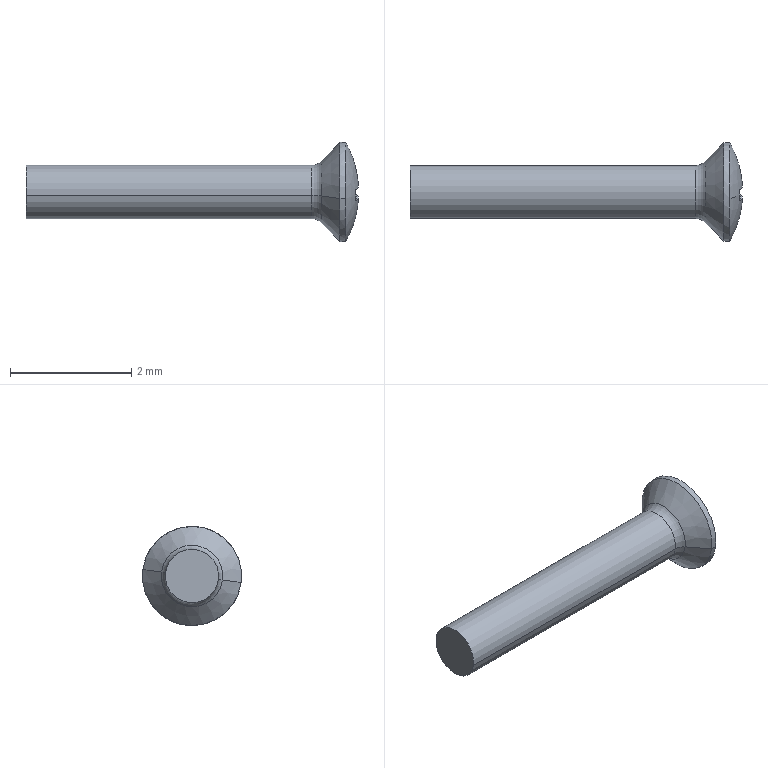Part | SolidWorks | features SplitBody 1 | 1 solid | 33 faces | box 5.48 x 1.637 x 1.637 mm | volume 3.726 mm3 | plane 17 | cone 8 | cylinder 4 | torus 2 | sphere 2 | commonest cylinder face diameters 0.88 x2 1.637 x2